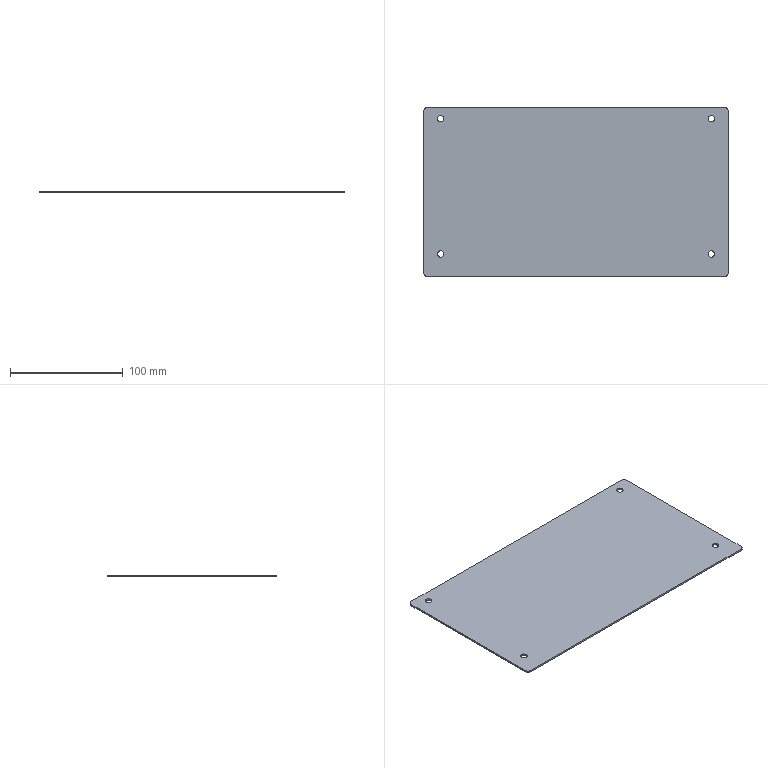Part | STEP file | J453-EBZ05-07-08-Part-1 | 1 solid | 18 faces | box 270 x 150 x 1.5 mm | volume 60580 mm3 | cylinder 12 | plane 6 | commonest cylinder face diameters 5.8 x8 6 x4